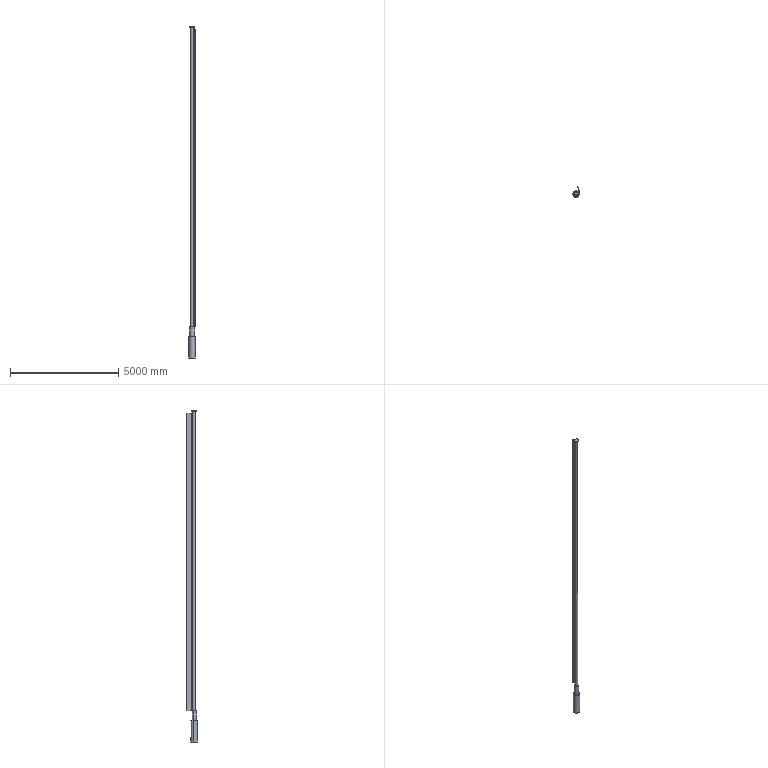Part | SolidWorks | features ICE 9, Extrusion 1 | 1 solid | 27 faces | box 300 x 474.612 x 15314 mm | volume 388904585 mm3 | plane 19 | cylinder 8 | commonest cylinder face diameters 200 x4 300 x2 100 x1 117.35 x1
STEP:
#1=CARTESIAN_POINT('',(-100.,0.,-14264.));
#2=VERTEX_POINT('',#1);
#3=CARTESIAN_POINT('',(100.,0.,-14264.));
#4=VERTEX_POINT('',#3);
#5=CARTESIAN_POINT('',(0.,0.,-14264.));
#6=DIRECTION('',(0.,0.,-1.));
#7=DIRECTION('',(-1.,0.,0.));
#8=AXIS2_PLACEMENT_3D('',#5,#6,#7);
#9=CIRCLE('',#8,100.);
#10=EDGE_CURVE('',#2,#4,#9,.T.);
#11=ORIENTED_EDGE('',*,*,#10,.F.);
#12=CARTESIAN_POINT('',(-100.,0.,-13824.));
#13=VERTEX_POINT('',#12);
#14=CARTESIAN_POINT('',(-100.,0.,-14264.));
#15=DIRECTION('',(0.,0.,1.));
#16=VECTOR('',#15,1000.);
#17=LINE('',#14,#16);
#18=EDGE_CURVE('',#2,#13,#17,.T.);
#19=ORIENTED_EDGE('',*,*,#18,.T.);
#20=CARTESIAN_POINT('',(61.826,78.598,-13824.));
#21=VERTEX_POINT('',#20);
#22=CARTESIAN_POINT('',(0.,0.,-13824.));
#23=DIRECTION('',(0.,0.,-1.));
#24=DIRECTION('',(-1.,0.,0.));
#25=AXIS2_PLACEMENT_3D('',#22,#23,#24);
#26=CIRCLE('',#25,100.);
#27=EDGE_CURVE('',#13,#21,#26,.T.);
#28=ORIENTED_EDGE('',*,*,#27,.T.);
#29=CARTESIAN_POINT('',(96.233,27.187,-13824.));
#30=VERTEX_POINT('',#29);
#31=CARTESIAN_POINT('',(0.,0.,-13824.));
#32=DIRECTION('',(0.,0.,-1.));
#33=DIRECTION('',(-1.,0.,0.));
#34=AXIS2_PLACEMENT_3D('',#31,#32,#33);
#35=CIRCLE('',#34,100.);
#36=EDGE_CURVE('',#21,#30,#35,.T.);
#37=ORIENTED_EDGE('',*,*,#36,.T.);
#38=CARTESIAN_POINT('',(100.,0.,-13824.));
#39=VERTEX_POINT('',#38);
#40=CARTESIAN_POINT('',(0.,0.,-13824.));
#41=DIRECTION('',(0.,0.,-1.));
#42=DIRECTION('',(-1.,0.,0.));
#43=AXIS2_PLACEMENT_3D('',#40,#41,#42);
#44=CIRCLE('',#43,100.);
#45=EDGE_CURVE('',#30,#39,#44,.T.);
#46=ORIENTED_EDGE('',*,*,#45,.T.);
#47=CARTESIAN_POINT('',(100.,0.,-14264.));
#48=DIRECTION('',(0.,0.,1.));
#49=VECTOR('',#48,1000.);
#50=LINE('',#47,#49);
#51=EDGE_CURVE('',#4,#39,#50,.T.);
#52=ORIENTED_EDGE('',*,*,#51,.F.);
#53=EDGE_LOOP('',(#11,#19,#28,#37,#46,#52));
#54=FACE_OUTER_BOUND('',#53,.T.);
#55=CARTESIAN_POINT('',(0.,0.,-14264.));
#56=DIRECTION('',(0.,0.,1.));
#57=DIRECTION('',(1.,0.,0.));
#58=AXIS2_PLACEMENT_3D('',#55,#56,#57);
#59=CYLINDRICAL_SURFACE('',#58,100.);
#60=ADVANCED_FACE('',(#54),#59,.T.);
#61=CARTESIAN_POINT('',(-100.,0.,50.));
#62=VERTEX_POINT('',#61);
#63=CARTESIAN_POINT('',(100.,0.,50.));
#64=VERTEX_POINT('',#63);
#65=CARTESIAN_POINT('',(0.,0.,50.));
#66=DIRECTION('',(0.,0.,-1.));
#67=DIRECTION('',(-1.,0.,0.));
#68=AXIS2_PLACEMENT_3D('',#65,#66,#67);
#69=CIRCLE('',#68,100.);
#70=EDGE_CURVE('',#62,#64,#69,.T.);
#71=ORIENTED_EDGE('',*,*,#70,.T.);
#72=CARTESIAN_POINT('',(100.,0.,0.));
#73=VERTEX_POINT('',#72);
#74=CARTESIAN_POINT('',(100.,0.,50.));
#75=DIRECTION('',(0.,0.,-1.));
#76=VECTOR('',#75,1000.);
#77=LINE('',#74,#76);
#78=EDGE_CURVE('',#64,#73,#77,.T.);
#79=ORIENTED_EDGE('',*,*,#78,.T.);
#80=CARTESIAN_POINT('',(96.233,27.187,0.));
#81=VERTEX_POINT('',#80);
#82=CARTESIAN_POINT('',(0.,0.,0.));
#83=DIRECTION('',(0.,0.,1.));
#84=DIRECTION('',(1.,0.,0.));
#85=AXIS2_PLACEMENT_3D('',#82,#83,#84);
#86=CIRCLE('',#85,100.);
#87=EDGE_CURVE('',#73,#81,#86,.T.);
#88=ORIENTED_EDGE('',*,*,#87,.T.);
#89=CARTESIAN_POINT('',(96.233,27.187,-100.));
#90=VERTEX_POINT('',#89);
#91=CARTESIAN_POINT('',(96.233,27.187,-100.));
#92=DIRECTION('',(0.,0.,1.));
#93=VECTOR('',#92,1000.);
#94=LINE('',#91,#93);
#95=EDGE_CURVE('',#90,#81,#94,.T.);
#96=ORIENTED_EDGE('',*,*,#95,.F.);
#97=CARTESIAN_POINT('',(61.826,78.598,-100.));
#98=VERTEX_POINT('',#97);
#99=CARTESIAN_POINT('',(0.,0.,-100.));
#100=DIRECTION('',(0.,0.,-1.));
#101=DIRECTION('',(1.,0.,0.));
#102=AXIS2_PLACEMENT_3D('',#99,#100,#101);
#103=CIRCLE('',#102,100.);
#104=EDGE_CURVE('',#98,#90,#103,.T.);
#105=ORIENTED_EDGE('',*,*,#104,.F.);
#106=CARTESIAN_POINT('',(61.826,78.598,0.));
#107=VERTEX_POINT('',#106);
#108=CARTESIAN_POINT('',(61.826,78.598,-100.));
#109=DIRECTION('',(0.,0.,1.));
#110=VECTOR('',#109,1000.);
#111=LINE('',#108,#110);
#112=EDGE_CURVE('',#98,#107,#111,.T.);
#113=ORIENTED_EDGE('',*,*,#112,.T.);
#114=CARTESIAN_POINT('',(-100.,0.,0.));
#115=VERTEX_POINT('',#114);
#116=CARTESIAN_POINT('',(0.,0.,0.));
#117=DIRECTION('',(0.,0.,1.));
#118=DIRECTION('',(1.,0.,0.));
#119=AXIS2_PLACEMENT_3D('',#116,#117,#118);
#120=CIRCLE('',#119,100.);
#121=EDGE_CURVE('',#107,#115,#120,.T.);
#122=ORIENTED_EDGE('',*,*,#121,.T.);
#123=CARTESIAN_POINT('',(-100.,0.,50.));
#124=DIRECTION('',(0.,0.,-1.));
#125=VECTOR('',#124,1000.);
#126=LINE('',#123,#125);
#127=EDGE_CURVE('',#62,#115,#126,.T.);
#128=ORIENTED_EDGE('',*,*,#127,.F.);
#129=EDGE_LOOP('',(#71,#79,#88,#96,#105,#113,#122,#128));
#130=FACE_OUTER_BOUND('',#129,.T.);
#131=CARTESIAN_POINT('',(0.,0.,50.));
#132=DIRECTION('',(0.,0.,-1.));
#133=DIRECTION('',(-1.,0.,0.));
#134=AXIS2_PLACEMENT_3D('',#131,#132,#133);
#135=CYLINDRICAL_SURFACE('',#134,100.);
#136=ADVANCED_FACE('',(#130),#135,.T.);
#137=CARTESIAN_POINT('',(-150.,0.,-15264.));
#138=VERTEX_POINT('',#137);
#139=CARTESIAN_POINT('',(-50.,141.421,-15264.));
#140=VERTEX_POINT('',#139);
#141=CARTESIAN_POINT('',(0.,0.,-15264.));
#142=DIRECTION('',(0.,0.,-1.));
#143=DIRECTION('',(-1.,0.,0.));
#144=AXIS2_PLACEMENT_3D('',#141,#142,#143);
#145=CIRCLE('',#144,150.);
#146=EDGE_CURVE('',#138,#140,#145,.T.);
#147=ORIENTED_EDGE('',*,*,#146,.F.);
#148=CARTESIAN_POINT('',(-150.,0.,-14264.));
#149=VERTEX_POINT('',#148);
#150=CARTESIAN_POINT('',(-150.,0.,-15264.));
#151=DIRECTION('',(0.,0.,1.));
#152=VECTOR('',#151,1000.);
#153=LINE('',#150,#152);
#154=EDGE_CURVE('',#138,#149,#153,.T.);
#155=ORIENTED_EDGE('',*,*,#154,.T.);
#156=CARTESIAN_POINT('',(150.,0.,-14264.));
#157=VERTEX_POINT('',#156);
#158=CARTESIAN_POINT('',(0.,0.,-14264.));
#159=DIRECTION('',(0.,0.,-1.));
#160=DIRECTION('',(-1.,0.,0.));
#161=AXIS2_PLACEMENT_3D('',#158,#159,#160);
#162=CIRCLE('',#161,150.);
#163=EDGE_CURVE('',#149,#157,#162,.T.);
#164=ORIENTED_EDGE('',*,*,#163,.T.);
#165=CARTESIAN_POINT('',(150.,0.,-15264.));
#166=VERTEX_POINT('',#165);
#167=CARTESIAN_POINT('',(150.,0.,-15264.));
#168=DIRECTION('',(0.,0.,1.));
#169=VECTOR('',#168,1000.);
#170=LINE('',#167,#169);
#171=EDGE_CURVE('',#166,#157,#170,.T.);
#172=ORIENTED_EDGE('',*,*,#171,.F.);
#173=CARTESIAN_POINT('',(50.,141.421,-15264.));
#174=VERTEX_POINT('',#173);
#175=CARTESIAN_POINT('',(0.,0.,-15264.));
#176=DIRECTION('',(0.,0.,-1.));
#177=DIRECTION('',(-1.,0.,0.));
#178=AXIS2_PLACEMENT_3D('',#175,#176,#177);
#179=CIRCLE('',#178,150.);
#180=EDGE_CURVE('',#174,#166,#179,.T.);
#181=ORIENTED_EDGE('',*,*,#180,.F.);
#182=CARTESIAN_POINT('',(50.,141.421,-15084.));
#183=VERTEX_POINT('',#182);
#184=CARTESIAN_POINT('',(50.,141.421,-15264.));
#185=DIRECTION('',(0.,0.,-1.));
#186=VECTOR('',#185,1000.);
#187=LINE('',#184,#186);
#188=EDGE_CURVE('',#183,#174,#187,.T.);
#189=ORIENTED_EDGE('',*,*,#188,.F.);
#190=CARTESIAN_POINT('',(-50.,141.421,-15084.));
#191=VERTEX_POINT('',#190);
#192=CARTESIAN_POINT('',(-50.,141.421,-15084.));
#193=CARTESIAN_POINT('',(-50.,141.421,-15080.672));
#194=CARTESIAN_POINT('',(-49.671,141.539,-15077.404));
#195=CARTESIAN_POINT('',(-48.708,141.872,-15072.589));
#196=CARTESIAN_POINT('',(-48.308,142.009,-15070.998));
#197=CARTESIAN_POINT('',(-47.588,142.251,-15068.634));
#198=CARTESIAN_POINT('',(-47.326,142.339,-15067.848));
#199=CARTESIAN_POINT('',(-46.768,142.523,-15066.297));
#200=CARTESIAN_POINT('',(-46.472,142.62,-15065.532));
#201=CARTESIAN_POINT('',(-44.899,143.129,-15061.757));
#202=CARTESIAN_POINT('',(-43.363,143.608,-15058.895));
#203=CARTESIAN_POINT('',(-41.098,144.261,-15055.511));
#204=CARTESIAN_POINT('',(-40.627,144.394,-15054.844));
#205=CARTESIAN_POINT('',(-39.651,144.665,-15053.529));
#206=CARTESIAN_POINT('',(-39.146,144.803,-15052.883));
#207=CARTESIAN_POINT('',(-37.593,145.217,-15050.994));
#208=CARTESIAN_POINT('',(-36.503,145.495,-15049.793));
#209=CARTESIAN_POINT('',(-33.072,146.328,-15046.361));
#210=CARTESIAN_POINT('',(-30.571,146.878,-15044.299));
#211=CARTESIAN_POINT('',(-26.479,147.651,-15041.555));
#212=CARTESIAN_POINT('',(-25.079,147.896,-15040.714));
#213=CARTESIAN_POINT('',(-22.212,148.353,-15039.175));
#214=CARTESIAN_POINT('',(-20.744,148.566,-15038.477));
#215=CARTESIAN_POINT('',(-17.741,148.955,-15037.225));
#216=CARTESIAN_POINT('',(-16.206,149.13,-15036.671));
#217=CARTESIAN_POINT('',(-13.849,149.361,-15035.949));
#218=CARTESIAN_POINT('',(-13.055,149.433,-15035.727));
#219=CARTESIAN_POINT('',(-11.448,149.565,-15035.321));
#220=CARTESIAN_POINT('',(-10.64,149.624,-15035.138));
#221=CARTESIAN_POINT('',(-6.6,149.89,-15034.328));
#222=CARTESIAN_POINT('',(-3.34,149.999,-15034.004));
#223=CARTESIAN_POINT('',(0.7688,150.,-15033.999));
#224=CARTESIAN_POINT('',(1.592,149.994,-15034.019));
#225=CARTESIAN_POINT('',(3.243,149.967,-15034.098));
#226=CARTESIAN_POINT('',(4.072,149.947,-15034.159));
#227=CARTESIAN_POINT('',(6.551,149.866,-15034.403));
#228=CARTESIAN_POINT('',(8.181,149.785,-15034.647));
#229=CARTESIAN_POINT('',(13.006,149.47,-15035.61));
#230=CARTESIAN_POINT('',(16.136,149.161,-15036.561));
#231=CARTESIAN_POINT('',(19.939,148.671,-15038.14));
#232=CARTESIAN_POINT('',(20.695,148.567,-15038.476));
#233=CARTESIAN_POINT('',(22.178,148.353,-15039.18));
#234=CARTESIAN_POINT('',(22.908,148.242,-15039.549));
#235=CARTESIAN_POINT('',(25.063,147.898,-15040.705));
#236=CARTESIAN_POINT('',(26.456,147.655,-15041.541));
#237=CARTESIAN_POINT('',(29.152,147.146,-15043.346));
#238=CARTESIAN_POINT('',(30.456,146.881,-15044.313));
#239=CARTESIAN_POINT('',(32.347,146.472,-15045.864));
#240=CARTESIAN_POINT('',(32.966,146.334,-15046.398));
#241=CARTESIAN_POINT('',(34.18,146.055,-15047.498));
#242=CARTESIAN_POINT('',(34.771,145.915,-15048.061));
#243=CARTESIAN_POINT('',(37.648,145.218,-15050.936));
#244=CARTESIAN_POINT('',(39.702,144.663,-15053.434));
#245=CARTESIAN_POINT('',(41.965,144.011,-15056.805));
#246=CARTESIAN_POINT('',(42.403,143.883,-15057.492));
#247=CARTESIAN_POINT('',(43.246,143.631,-15058.892));
#248=CARTESIAN_POINT('',(43.653,143.508,-15059.606));
#249=CARTESIAN_POINT('',(44.82,143.15,-15061.777));
#250=CARTESIAN_POINT('',(45.522,142.927,-15063.253));
#251=CARTESIAN_POINT('',(47.402,142.319,-15067.763));
#252=CARTESIAN_POINT('',(48.361,141.992,-15070.88));
#253=CARTESIAN_POINT('',(49.176,141.71,-15074.922));
#254=CARTESIAN_POINT('',(49.32,141.66,-15075.739));
#255=CARTESIAN_POINT('',(49.567,141.574,-15077.381));
#256=CARTESIAN_POINT('',(49.67,141.538,-15078.204));
#257=CARTESIAN_POINT('',(49.917,141.451,-15080.679));
#258=CARTESIAN_POINT('',(50.,141.421,-15082.336));
#259=CARTESIAN_POINT('',(50.,141.421,-15084.));
#260=B_SPLINE_CURVE_WITH_KNOTS('',3,(#192,#193,#194,#195,#196,#197,#198,#199,#200,#201,#202,#203,#204,#205,#206,#207,#208,#209,#210,#211,#212,#213,#214,#215,#216,#217,#218,#219,#220,#221,#222,#223,#224,#225,#226,#227,#228,#229,#230,#231,#232,#233,#234,#235,#236,#237,#238,#239,#240,#241,#242,#243,#244,#245,#246,#247,#248,#249,#250,#251,#252,#253,#254,#255,#256,#257,#258,#259),.UNSPECIFIED.,.F.,.F.,(4,2,2,2,2,2,2,2,2,2,2,2,2,2,2,2,2,2,2,2,2,2,2,2,2,2,2,2,2,2,2,2,2,4),(0.,0.009837,0.01476,0.01721,0.01967,0.02951,0.03197,0.03443,0.03935,0.04919,0.0541,0.05902,0.06394,0.0664,0.06886,0.0787,0.08116,0.08362,0.08853,0.09837,0.1008,0.1033,0.1082,0.1131,0.1156,0.118,0.1279,0.1303,0.1328,0.1377,0.1476,0.15,0.1525,0.1574),.UNSPECIFIED.);
#261=EDGE_CURVE('',#191,#183,#260,.T.);
#262=ORIENTED_EDGE('',*,*,#261,.F.);
#263=CARTESIAN_POINT('',(-50.,141.421,-15264.));
#264=DIRECTION('',(0.,0.,1.));
#265=VECTOR('',#264,1000.);
#266=LINE('',#263,#265);
#267=EDGE_CURVE('',#140,#191,#266,.T.);
#268=ORIENTED_EDGE('',*,*,#267,.F.);
#269=EDGE_LOOP('',(#147,#155,#164,#172,#181,#189,#262,#268));
#270=FACE_OUTER_BOUND('',#269,.T.);
#271=CARTESIAN_POINT('',(0.,0.,-15264.));
#272=DIRECTION('',(0.,0.,1.));
#273=DIRECTION('',(1.,0.,0.));
#274=AXIS2_PLACEMENT_3D('',#271,#272,#273);
#275=CYLINDRICAL_SURFACE('',#274,150.);
#276=ADVANCED_FACE('',(#270),#275,.T.);
#277=ORIENTED_EDGE('',*,*,#154,.F.);
#278=CARTESIAN_POINT('',(0.,0.,-15264.));
#279=DIRECTION('',(0.,0.,-1.));
#280=DIRECTION('',(-1.,0.,0.));
#281=AXIS2_PLACEMENT_3D('',#278,#279,#280);
#282=CIRCLE('',#281,150.);
#283=EDGE_CURVE('',#166,#138,#282,.T.);
#284=ORIENTED_EDGE('',*,*,#283,.F.);
#285=ORIENTED_EDGE('',*,*,#171,.T.);
#286=CARTESIAN_POINT('',(0.,0.,-14264.));
#287=DIRECTION('',(0.,0.,-1.));
#288=DIRECTION('',(-1.,0.,0.));
#289=AXIS2_PLACEMENT_3D('',#286,#287,#288);
#290=CIRCLE('',#289,150.);
#291=EDGE_CURVE('',#157,#149,#290,.T.);
#292=ORIENTED_EDGE('',*,*,#291,.T.);
#293=EDGE_LOOP('',(#277,#284,#285,#292));
#294=FACE_OUTER_BOUND('',#293,.T.);
#295=CARTESIAN_POINT('',(0.,0.,-15264.));
#296=DIRECTION('',(0.,0.,1.));
#297=DIRECTION('',(1.,0.,0.));
#298=AXIS2_PLACEMENT_3D('',#295,#296,#297);
#299=CYLINDRICAL_SURFACE('',#298,150.);
#300=ADVANCED_FACE('',(#294),#299,.T.);
#301=ORIENTED_EDGE('',*,*,#180,.T.);
#302=ORIENTED_EDGE('',*,*,#283,.T.);
#303=ORIENTED_EDGE('',*,*,#146,.T.);
#304=CARTESIAN_POINT('',(-50.,65.,-15264.));
#305=VERTEX_POINT('',#304);
#306=CARTESIAN_POINT('',(-50.,0.,-15264.));
#307=DIRECTION('',(0.,-1.,0.));
#308=VECTOR('',#307,1000.);
#309=LINE('',#306,#308);
#310=EDGE_CURVE('',#140,#305,#309,.T.);
#311=ORIENTED_EDGE('',*,*,#310,.T.);
#312=CARTESIAN_POINT('',(50.,65.,-15264.));
#313=VERTEX_POINT('',#312);
#314=CARTESIAN_POINT('',(0.,65.,-15264.));
#315=DIRECTION('',(1.,0.,0.));
#316=VECTOR('',#315,1000.);
#317=LINE('',#314,#316);
#318=EDGE_CURVE('',#305,#313,#317,.T.);
#319=ORIENTED_EDGE('',*,*,#318,.T.);
#320=CARTESIAN_POINT('',(50.,0.,-15264.));
#321=DIRECTION('',(0.,1.,0.));
#322=VECTOR('',#321,1000.);
#323=LINE('',#320,#322);
#324=EDGE_CURVE('',#313,#174,#323,.T.);
#325=ORIENTED_EDGE('',*,*,#324,.T.);
#326=EDGE_LOOP('',(#301,#302,#303,#311,#319,#325));
#327=FACE_OUTER_BOUND('',#326,.T.);
#328=CARTESIAN_POINT('',(0.,0.,-15264.));
#329=DIRECTION('',(0.,0.,-1.));
#330=DIRECTION('',(-1.,0.,0.));
#331=AXIS2_PLACEMENT_3D('',#328,#329,#330);
#332=PLANE('',#331);
#333=ADVANCED_FACE('',(#327),#332,.T.);
#334=CARTESIAN_POINT('',(127.239,110.96,-100.));
#335=VERTEX_POINT('',#334);
#336=CARTESIAN_POINT('',(127.239,110.96,-100.));
#337=DIRECTION('',(-0.8963,-0.4434,0.));
#338=VECTOR('',#337,1000.);
#339=LINE('',#336,#338);
#340=EDGE_CURVE('',#335,#98,#339,.T.);
#341=ORIENTED_EDGE('',*,*,#340,.F.);
#342=CARTESIAN_POINT('',(127.239,110.96,-13824.));
#343=VERTEX_POINT('',#342);
#344=CARTESIAN_POINT('',(127.239,110.96,-13824.));
#345=DIRECTION('',(0.,0.,1.));
#346=VECTOR('',#345,1000.);
#347=LINE('',#344,#346);
#348=EDGE_CURVE('',#343,#335,#347,.T.);
#349=ORIENTED_EDGE('',*,*,#348,.F.);
#350=CARTESIAN_POINT('',(127.239,110.96,-13824.));
#351=DIRECTION('',(0.8963,0.4434,0.));
#352=VECTOR('',#351,1000.);
#353=LINE('',#350,#352);
#354=EDGE_CURVE('',#21,#343,#353,.T.);
#355=ORIENTED_EDGE('',*,*,#354,.F.);
#356=CARTESIAN_POINT('',(61.826,78.598,-13824.));
#357=DIRECTION('',(0.,0.,1.));
#358=VECTOR('',#357,1000.);
#359=LINE('',#356,#358);
#360=EDGE_CURVE('',#21,#98,#359,.T.);
#361=ORIENTED_EDGE('',*,*,#360,.T.);
#362=EDGE_LOOP('',(#341,#349,#355,#361));
#363=FACE_OUTER_BOUND('',#362,.T.);
#364=CARTESIAN_POINT('',(127.239,110.96,-13824.));
#365=DIRECTION('',(0.4434,-0.8963,0.));
#366=DIRECTION('',(0.8963,0.4434,0.));
#367=AXIS2_PLACEMENT_3D('',#364,#365,#366);
#368=PLANE('',#367);
#369=ADVANCED_FACE('',(#363),#368,.F.);
#370=CARTESIAN_POINT('',(106.547,286.808,-100.));
#371=VERTEX_POINT('',#370);
#372=CARTESIAN_POINT('',(106.547,286.808,-100.));
#373=DIRECTION('',(0.1169,-0.9931,0.));
#374=VECTOR('',#373,1000.);
#375=LINE('',#372,#374);
#376=EDGE_CURVE('',#371,#335,#375,.T.);
#377=ORIENTED_EDGE('',*,*,#376,.F.);
#378=CARTESIAN_POINT('',(106.547,286.808,-13824.));
#379=VERTEX_POINT('',#378);
#380=CARTESIAN_POINT('',(106.547,286.808,-13824.));
#381=DIRECTION('',(0.,0.,1.));
#382=VECTOR('',#381,1000.);
#383=LINE('',#380,#382);
#384=EDGE_CURVE('',#379,#371,#383,.T.);
#385=ORIENTED_EDGE('',*,*,#384,.F.);
#386=CARTESIAN_POINT('',(106.547,286.808,-13824.));
#387=DIRECTION('',(-0.1169,0.9931,0.));
#388=VECTOR('',#387,1000.);
#389=LINE('',#386,#388);
#390=EDGE_CURVE('',#343,#379,#389,.T.);
#391=ORIENTED_EDGE('',*,*,#390,.F.);
#392=ORIENTED_EDGE('',*,*,#348,.T.);
#393=EDGE_LOOP('',(#377,#385,#391,#392));
#394=FACE_OUTER_BOUND('',#393,.T.);
#395=CARTESIAN_POINT('',(106.547,286.808,-13824.));
#396=DIRECTION('',(0.9931,0.1169,0.));
#397=DIRECTION('',(-0.1169,0.9931,0.));
#398=AXIS2_PLACEMENT_3D('',#395,#396,#397);
#399=PLANE('',#398);
#400=ADVANCED_FACE('',(#394),#399,.F.);
#401=CARTESIAN_POINT('',(53.816,324.612,-100.));
#402=VERTEX_POINT('',#401);
#403=CARTESIAN_POINT('',(53.816,324.612,-100.));
#404=DIRECTION('',(0.8127,-0.5827,0.));
#405=VECTOR('',#404,1000.);
#406=LINE('',#403,#405);
#407=EDGE_CURVE('',#402,#371,#406,.T.);
#408=ORIENTED_EDGE('',*,*,#407,.F.);
#409=CARTESIAN_POINT('',(53.816,324.612,-13824.));
#410=VERTEX_POINT('',#409);
#411=CARTESIAN_POINT('',(53.816,324.612,-13824.));
#412=DIRECTION('',(0.,0.,1.));
#413=VECTOR('',#412,1000.);
#414=LINE('',#411,#413);
#415=EDGE_CURVE('',#410,#402,#414,.T.);
#416=ORIENTED_EDGE('',*,*,#415,.F.);
#417=CARTESIAN_POINT('',(69.836,313.127,-13824.));
#418=DIRECTION('',(-0.8127,0.5827,0.));
#419=VECTOR('',#418,1000.);
#420=LINE('',#417,#419);
#421=EDGE_CURVE('',#379,#410,#420,.T.);
#422=ORIENTED_EDGE('',*,*,#421,.F.);
#423=ORIENTED_EDGE('',*,*,#384,.T.);
#424=EDGE_LOOP('',(#408,#416,#422,#423));
#425=FACE_OUTER_BOUND('',#424,.T.);
#426=CARTESIAN_POINT('',(53.816,324.612,-13824.));
#427=DIRECTION('',(0.5827,0.8127,0.));
#428=DIRECTION('',(-0.8127,0.5827,0.));
#429=AXIS2_PLACEMENT_3D('',#426,#427,#428);
#430=PLANE('',#429);
#431=ADVANCED_FACE('',(#425),#430,.F.);
#432=CARTESIAN_POINT('',(85.855,324.612,-100.));
#433=VERTEX_POINT('',#432);
#434=CARTESIAN_POINT('',(85.855,324.612,-100.));
#435=DIRECTION('',(-1.,0.,0.));
#436=VECTOR('',#435,1000.);
#437=LINE('',#434,#436);
#438=EDGE_CURVE('',#433,#402,#437,.T.);
#439=ORIENTED_EDGE('',*,*,#438,.F.);
#440=CARTESIAN_POINT('',(85.855,324.612,-13824.));
#441=VERTEX_POINT('',#440);
#442=CARTESIAN_POINT('',(85.855,324.612,-13824.));
#443=DIRECTION('',(0.,0.,1.));
#444=VECTOR('',#443,1000.);
#445=LINE('',#442,#444);
#446=EDGE_CURVE('',#441,#433,#445,.T.);
#447=ORIENTED_EDGE('',*,*,#446,.F.);
#448=CARTESIAN_POINT('',(85.855,324.612,-13824.));
#449=DIRECTION('',(1.,0.,0.));
#450=VECTOR('',#449,1000.);
#451=LINE('',#448,#450);
#452=EDGE_CURVE('',#410,#441,#451,.T.);
#453=ORIENTED_EDGE('',*,*,#452,.F.);
#454=ORIENTED_EDGE('',*,*,#415,.T.);
#455=EDGE_LOOP('',(#439,#447,#453,#454));
#456=FACE_OUTER_BOUND('',#455,.T.);
#457=CARTESIAN_POINT('',(85.855,324.612,-13824.));
#458=DIRECTION('',(0.,-1.,0.));
#459=DIRECTION('',(0.,0.,-1.));
#460=AXIS2_PLACEMENT_3D('',#457,#458,#459);
#461=PLANE('',#460);
#462=ADVANCED_FACE('',(#456),#461,.F.);
#463=CARTESIAN_POINT('',(127.239,294.943,-100.));
#464=VERTEX_POINT('',#463);
#465=CARTESIAN_POINT('',(127.239,294.943,-100.));
#466=DIRECTION('',(-0.8127,0.5827,0.));
#467=VECTOR('',#466,1000.);
#468=LINE('',#465,#467);
#469=EDGE_CURVE('',#464,#433,#468,.T.);
#470=ORIENTED_EDGE('',*,*,#469,.F.);
#471=CARTESIAN_POINT('',(127.239,294.943,-13824.));
#472=VERTEX_POINT('',#471);
#473=CARTESIAN_POINT('',(127.239,294.943,-13824.));
#474=DIRECTION('',(0.,0.,1.));
#475=VECTOR('',#474,1000.);
#476=LINE('',#473,#475);
#477=EDGE_CURVE('',#472,#464,#476,.T.);
#478=ORIENTED_EDGE('',*,*,#477,.F.);
#479=CARTESIAN_POINT('',(127.239,294.943,-13824.));
#480=DIRECTION('',(0.8127,-0.5827,0.));
#481=VECTOR('',#480,1000.);
#482=LINE('',#479,#481);
#483=EDGE_CURVE('',#441,#472,#482,.T.);
#484=ORIENTED_EDGE('',*,*,#483,.F.);
#485=ORIENTED_EDGE('',*,*,#446,.T.);
#486=EDGE_LOOP('',(#470,#478,#484,#485));
#487=FACE_OUTER_BOUND('',#486,.T.);
#488=CARTESIAN_POINT('',(127.239,294.943,-13824.));
#489=DIRECTION('',(-0.5827,-0.8127,0.));
#490=DIRECTION('',(0.8127,-0.5827,0.));
#491=AXIS2_PLACEMENT_3D('',#488,#489,#490);
#492=PLANE('',#491);
#493=ADVANCED_FACE('',(#487),#492,.F.);
#494=CARTESIAN_POINT('',(146.429,97.202,-100.));
#495=VERTEX_POINT('',#494);
#496=CARTESIAN_POINT('',(146.429,97.202,-100.));
#497=DIRECTION('',(-0.09659,0.9953,0.));
#498=VECTOR('',#497,1000.);
#499=LINE('',#496,#498);
#500=EDGE_CURVE('',#495,#464,#499,.T.);
#501=ORIENTED_EDGE('',*,*,#500,.F.);
#502=CARTESIAN_POINT('',(146.429,97.202,-13824.));
#503=VERTEX_POINT('',#502);
#504=CARTESIAN_POINT('',(146.429,97.202,-13824.));
#505=DIRECTION('',(0.,0.,1.));
#506=VECTOR('',#505,1000.);
#507=LINE('',#504,#506);
#508=EDGE_CURVE('',#503,#495,#507,.T.);
#509=ORIENTED_EDGE('',*,*,#508,.F.);
#510=CARTESIAN_POINT('',(146.429,97.202,-13824.));
#511=DIRECTION('',(0.09659,-0.9953,0.));
#512=VECTOR('',#511,1000.);
#513=LINE('',#510,#512);
#514=EDGE_CURVE('',#472,#503,#513,.T.);
#515=ORIENTED_EDGE('',*,*,#514,.F.);
#516=ORIENTED_EDGE('',*,*,#477,.T.);
#517=EDGE_LOOP('',(#501,#509,#515,#516));
#518=FACE_OUTER_BOUND('',#517,.T.);
#519=CARTESIAN_POINT('',(146.429,97.202,-13824.));
#520=DIRECTION('',(-0.9953,-0.09659,0.));
#521=DIRECTION('',(0.09659,-0.9953,0.));
#522=AXIS2_PLACEMENT_3D('',#519,#520,#521);
#523=PLANE('',#522);
#524=ADVANCED_FACE('',(#518),#523,.F.);
#525=CARTESIAN_POINT('',(96.233,27.187,-100.));
#526=DIRECTION('',(0.5827,0.8127,0.));
#527=VECTOR('',#526,1000.);
#528=LINE('',#525,#527);
#529=EDGE_CURVE('',#90,#495,#528,.T.);
#530=ORIENTED_EDGE('',*,*,#529,.F.);
#531=CARTESIAN_POINT('',(96.233,27.187,-13824.));
#532=DIRECTION('',(0.,0.,1.));
#533=VECTOR('',#532,1000.);
#534=LINE('',#531,#533);
#535=EDGE_CURVE('',#30,#90,#534,.T.);
#536=ORIENTED_EDGE('',*,*,#535,.F.);
#537=CARTESIAN_POINT('',(96.233,27.187,-13824.));
#538=DIRECTION('',(-0.5827,-0.8127,0.));
#539=VECTOR('',#538,1000.);
#540=LINE('',#537,#539);
#541=EDGE_CURVE('',#503,#30,#540,.T.);
#542=ORIENTED_EDGE('',*,*,#541,.F.);
#543=ORIENTED_EDGE('',*,*,#508,.T.);
#544=EDGE_LOOP('',(#530,#536,#542,#543));
#545=FACE_OUTER_BOUND('',#544,.T.);
#546=CARTESIAN_POINT('',(96.233,27.187,-13824.));
#547=DIRECTION('',(-0.8127,0.5827,0.));
#548=DIRECTION('',(-0.5827,-0.8127,0.));
#549=AXIS2_PLACEMENT_3D('',#546,#547,#548);
#550=PLANE('',#549);
#551=ADVANCED_FACE('',(#545),#550,.F.);
#552=ORIENTED_EDGE('',*,*,#78,.F.);
#553=CARTESIAN_POINT('',(0.,0.,50.));
#554=DIRECTION('',(0.,0.,-1.));
#555=DIRECTION('',(-1.,0.,0.));
#556=AXIS2_PLACEMENT_3D('',#553,#554,#555);
#557=CIRCLE('',#556,100.);
#558=EDGE_CURVE('',#64,#62,#557,.T.);
#559=ORIENTED_EDGE('',*,*,#558,.T.);
#560=ORIENTED_EDGE('',*,*,#127,.T.);
#561=CARTESIAN_POINT('',(0.,0.,0.));
#562=DIRECTION('',(0.,0.,1.));
#563=DIRECTION('',(1.,0.,0.));
#564=AXIS2_PLACEMENT_3D('',#561,#562,#563);
#565=CIRCLE('',#564,100.);
#566=EDGE_CURVE('',#115,#73,#565,.T.);
#567=ORIENTED_EDGE('',*,*,#566,.T.);
#568=EDGE_LOOP('',(#552,#559,#560,#567));
#569=FACE_OUTER_BOUND('',#568,.T.);
#570=CARTESIAN_POINT('',(0.,0.,50.));
#571=DIRECTION('',(0.,0.,-1.));
#572=DIRECTION('',(-1.,0.,0.));
#573=AXIS2_PLACEMENT_3D('',#570,#571,#572);
#574=CYLINDRICAL_SURFACE('',#573,100.);
#575=ADVANCED_FACE('',(#569),#574,.T.);
#576=CARTESIAN_POINT('',(48.187,-33.477,0.));
#577=VERTEX_POINT('',#576);
#578=CARTESIAN_POINT('',(96.233,27.187,0.));
#579=DIRECTION('',(-0.6209,-0.7839,0.));
#580=VECTOR('',#579,1000.);
#581=LINE('',#578,#580);
#582=EDGE_CURVE('',#81,#577,#581,.T.);
#583=ORIENTED_EDGE('',*,*,#582,.F.);
#584=ORIENTED_EDGE('',*,*,#87,.F.);
#585=ORIENTED_EDGE('',*,*,#566,.F.);
#586=ORIENTED_EDGE('',*,*,#121,.F.);
#587=CARTESIAN_POINT('',(0.,58.675,0.));
#588=VERTEX_POINT('',#587);
#589=CARTESIAN_POINT('',(61.826,78.598,0.));
#590=DIRECTION('',(0.9518,0.3067,0.));
#591=VECTOR('',#590,1000.);
#592=LINE('',#589,#591);
#593=EDGE_CURVE('',#588,#107,#592,.T.);
#594=ORIENTED_EDGE('',*,*,#593,.F.);
#595=CARTESIAN_POINT('',(0.,0.,0.));
#596=DIRECTION('',(0.,0.,-1.));
#597=DIRECTION('',(-1.,0.,0.));
#598=AXIS2_PLACEMENT_3D('',#595,#596,#597);
#599=CIRCLE('',#598,58.675);
#600=EDGE_CURVE('',#577,#588,#599,.T.);
#601=ORIENTED_EDGE('',*,*,#600,.F.);
#602=EDGE_LOOP('',(#583,#584,#585,#586,#594,#601));
#603=FACE_OUTER_BOUND('',#602,.T.);
#604=CARTESIAN_POINT('',(0.,0.,0.));
#605=DIRECTION('',(0.,0.,1.));
#606=DIRECTION('',(1.,0.,0.));
#607=AXIS2_PLACEMENT_3D('',#604,#605,#606);
#608=PLANE('',#607);
#609=ADVANCED_FACE('',(#603),#608,.F.);
#610=ORIENTED_EDGE('',*,*,#582,.T.);
#611=CARTESIAN_POINT('',(48.187,-33.477,-13824.));
#612=VERTEX_POINT('',#611);
#613=CARTESIAN_POINT('',(48.187,-33.477,-13824.));
#614=DIRECTION('',(0.,0.,1.));
#615=VECTOR('',#614,1000.);
#616=LINE('',#613,#615);
#617=EDGE_CURVE('',#612,#577,#616,.T.);
#618=ORIENTED_EDGE('',*,*,#617,.F.);
#619=CARTESIAN_POINT('',(96.233,27.187,-13824.));
#620=DIRECTION('',(-0.6209,-0.7839,0.));
#621=VECTOR('',#620,1000.);
#622=LINE('',#619,#621);
#623=EDGE_CURVE('',#30,#612,#622,.T.);
#624=ORIENTED_EDGE('',*,*,#623,.F.);
#625=ORIENTED_EDGE('',*,*,#535,.T.);
#626=ORIENTED_EDGE('',*,*,#95,.T.);
#627=EDGE_LOOP('',(#610,#618,#624,#625,#626));
#628=FACE_OUTER_BOUND('',#627,.T.);
#629=CARTESIAN_POINT('',(96.233,27.187,-13824.));
#630=DIRECTION('',(-0.7839,0.6209,0.));
#631=DIRECTION('',(-0.6209,-0.7839,0.));
#632=AXIS2_PLACEMENT_3D('',#629,#630,#631);
#633=PLANE('',#632);
#634=ADVANCED_FACE('',(#628),#633,.F.);
#635=ORIENTED_EDGE('',*,*,#600,.T.);
#636=CARTESIAN_POINT('',(0.,58.675,-13824.));
#637=VERTEX_POINT('',#636);
#638=CARTESIAN_POINT('',(0.,58.675,-13824.));
#639=DIRECTION('',(0.,0.,1.));
#640=VECTOR('',#639,1000.);
#641=LINE('',#638,#640);
#642=EDGE_CURVE('',#637,#588,#641,.T.);
#643=ORIENTED_EDGE('',*,*,#642,.F.);
#644=CARTESIAN_POINT('',(0.,0.,-13824.));
#645=DIRECTION('',(0.,0.,-1.));
#646=DIRECTION('',(-1.,0.,0.));
#647=AXIS2_PLACEMENT_3D('',#644,#645,#646);
#648=CIRCLE('',#647,58.675);
#649=EDGE_CURVE('',#612,#637,#648,.T.);
#650=ORIENTED_EDGE('',*,*,#649,.F.);
#651=ORIENTED_EDGE('',*,*,#617,.T.);
#652=EDGE_LOOP('',(#635,#643,#650,#651));
#653=FACE_OUTER_BOUND('',#652,.T.);
#654=CARTESIAN_POINT('',(0.,0.,-13824.));
#655=DIRECTION('',(0.,0.,1.));
#656=DIRECTION('',(1.,0.,0.));
#657=AXIS2_PLACEMENT_3D('',#654,#655,#656);
#658=CYLINDRICAL_SURFACE('',#657,58.675);
#659=ADVANCED_FACE('',(#653),#658,.T.);
#660=ORIENTED_EDGE('',*,*,#593,.T.);
#661=ORIENTED_EDGE('',*,*,#112,.F.);
#662=ORIENTED_EDGE('',*,*,#360,.F.);
#663=CARTESIAN_POINT('',(61.826,78.598,-13824.));
#664=DIRECTION('',(0.9518,0.3067,0.));
#665=VECTOR('',#664,1000.);
#666=LINE('',#663,#665);
#667=EDGE_CURVE('',#637,#21,#666,.T.);
#668=ORIENTED_EDGE('',*,*,#667,.F.);
#669=ORIENTED_EDGE('',*,*,#642,.T.);
#670=EDGE_LOOP('',(#660,#661,#662,#668,#669));
#671=FACE_OUTER_BOUND('',#670,.T.);
#672=CARTESIAN_POINT('',(61.826,78.598,-13824.));
#673=DIRECTION('',(0.3067,-0.9518,0.));
#674=DIRECTION('',(0.9518,0.3067,0.));
#675=AXIS2_PLACEMENT_3D('',#672,#673,#674);
#676=PLANE('',#675);
#677=ADVANCED_FACE('',(#671),#676,.F.);
#678=ORIENTED_EDGE('',*,*,#36,.F.);
#679=ORIENTED_EDGE('',*,*,#354,.T.);
#680=ORIENTED_EDGE('',*,*,#390,.T.);
#681=ORIENTED_EDGE('',*,*,#421,.T.);
#682=ORIENTED_EDGE('',*,*,#452,.T.);
#683=ORIENTED_EDGE('',*,*,#483,.T.);
#684=ORIENTED_EDGE('',*,*,#514,.T.);
#685=ORIENTED_EDGE('',*,*,#541,.T.);
#686=EDGE_LOOP('',(#678,#679,#680,#681,#682,#683,#684,#685));
#687=FACE_OUTER_BOUND('',#686,.T.);
#688=CARTESIAN_POINT('',(0.,0.,-13824.));
#689=DIRECTION('',(0.,0.,-1.));
#690=DIRECTION('',(-1.,0.,0.));
#691=AXIS2_PLACEMENT_3D('',#688,#689,#690);
#692=PLANE('',#691);
#693=ADVANCED_FACE('',(#687),#692,.T.);
#694=ORIENTED_EDGE('',*,*,#45,.F.);
#695=ORIENTED_EDGE('',*,*,#623,.T.);
#696=ORIENTED_EDGE('',*,*,#649,.T.);
#697=ORIENTED_EDGE('',*,*,#667,.T.);
#698=ORIENTED_EDGE('',*,*,#27,.F.);
#699=CARTESIAN_POINT('',(0.,0.,-13824.));
#700=DIRECTION('',(0.,0.,-1.));
#701=DIRECTION('',(-1.,0.,0.));
#702=AXIS2_PLACEMENT_3D('',#699,#700,#701);
#703=CIRCLE('',#702,100.);
#704=EDGE_CURVE('',#39,#13,#703,.T.);
#705=ORIENTED_EDGE('',*,*,#704,.F.);
#706=EDGE_LOOP('',(#694,#695,#696,#697,#698,#705));
#707=FACE_OUTER_BOUND('',#706,.T.);
#708=CARTESIAN_POINT('',(0.,0.,-13824.));
#709=DIRECTION('',(0.,0.,-1.));
#710=DIRECTION('',(-1.,0.,0.));
#711=AXIS2_PLACEMENT_3D('',#708,#709,#710);
#712=PLANE('',#711);
#713=ADVANCED_FACE('',(#707),#712,.F.);
#714=ORIENTED_EDGE('',*,*,#18,.F.);
#715=CARTESIAN_POINT('',(0.,0.,-14264.));
#716=DIRECTION('',(0.,0.,-1.));
#717=DIRECTION('',(-1.,0.,0.));
#718=AXIS2_PLACEMENT_3D('',#715,#716,#717);
#719=CIRCLE('',#718,100.);
#720=EDGE_CURVE('',#4,#2,#719,.T.);
#721=ORIENTED_EDGE('',*,*,#720,.F.);
#722=ORIENTED_EDGE('',*,*,#51,.T.);
#723=ORIENTED_EDGE('',*,*,#704,.T.);
#724=EDGE_LOOP('',(#714,#721,#722,#723));
#725=FACE_OUTER_BOUND('',#724,.T.);
#726=CARTESIAN_POINT('',(0.,0.,-14264.));
#727=DIRECTION('',(0.,0.,1.));
#728=DIRECTION('',(1.,0.,0.));
#729=AXIS2_PLACEMENT_3D('',#726,#727,#728);
#730=CYLINDRICAL_SURFACE('',#729,100.);
#731=ADVANCED_FACE('',(#725),#730,.T.);
#732=ORIENTED_EDGE('',*,*,#104,.T.);
#733=ORIENTED_EDGE('',*,*,#529,.T.);
#734=ORIENTED_EDGE('',*,*,#500,.T.);
#735=ORIENTED_EDGE('',*,*,#469,.T.);
#736=ORIENTED_EDGE('',*,*,#438,.T.);
#737=ORIENTED_EDGE('',*,*,#407,.T.);
#738=ORIENTED_EDGE('',*,*,#376,.T.);
#739=ORIENTED_EDGE('',*,*,#340,.T.);
#740=EDGE_LOOP('',(#732,#733,#734,#735,#736,#737,#738,#739));
#741=FACE_OUTER_BOUND('',#740,.T.);
#742=CARTESIAN_POINT('',(0.,0.,-100.));
#743=DIRECTION('',(0.,0.,1.));
#744=DIRECTION('',(1.,0.,0.));
#745=AXIS2_PLACEMENT_3D('',#742,#743,#744);
#746=PLANE('',#745);
#747=ADVANCED_FACE('',(#741),#746,.T.);
#748=ORIENTED_EDGE('',*,*,#720,.T.);
#749=ORIENTED_EDGE('',*,*,#10,.T.);
#750=EDGE_LOOP('',(#748,#749));
#751=FACE_BOUND('',#750,.T.);
#752=ORIENTED_EDGE('',*,*,#291,.F.);
#753=ORIENTED_EDGE('',*,*,#163,.F.);
#754=EDGE_LOOP('',(#752,#753));
#755=FACE_OUTER_BOUND('',#754,.T.);
#756=CARTESIAN_POINT('',(0.,0.,-14264.));
#757=DIRECTION('',(0.,0.,-1.));
#758=DIRECTION('',(-1.,0.,0.));
#759=AXIS2_PLACEMENT_3D('',#756,#757,#758);
#760=PLANE('',#759);
#761=ADVANCED_FACE('',(#751,#755),#760,.F.);
#762=ORIENTED_EDGE('',*,*,#261,.T.);
#763=CARTESIAN_POINT('',(50.,65.,-15084.));
#764=VERTEX_POINT('',#763);
#765=CARTESIAN_POINT('',(50.,365.,-15084.));
#766=DIRECTION('',(0.,-1.,0.));
#767=VECTOR('',#766,1000.);
#768=LINE('',#765,#767);
#769=EDGE_CURVE('',#183,#764,#768,.T.);
#770=ORIENTED_EDGE('',*,*,#769,.T.);
#771=CARTESIAN_POINT('',(-50.,65.,-15084.));
#772=VERTEX_POINT('',#771);
#773=CARTESIAN_POINT('',(0.,65.,-15084.));
#774=DIRECTION('',(0.,1.,0.));
#775=DIRECTION('',(0.,0.,1.));
#776=AXIS2_PLACEMENT_3D('',#773,#774,#775);
#777=CIRCLE('',#776,50.);
#778=EDGE_CURVE('',#772,#764,#777,.T.);
#779=ORIENTED_EDGE('',*,*,#778,.F.);
#780=CARTESIAN_POINT('',(-50.,365.,-15084.));
#781=DIRECTION('',(0.,-1.,0.));
#782=VECTOR('',#781,1000.);
#783=LINE('',#780,#782);
#784=EDGE_CURVE('',#191,#772,#783,.T.);
#785=ORIENTED_EDGE('',*,*,#784,.F.);
#786=EDGE_LOOP('',(#762,#770,#779,#785));
#787=FACE_OUTER_BOUND('',#786,.T.);
#788=CARTESIAN_POINT('',(0.,365.,-15084.));
#789=DIRECTION('',(0.,-1.,0.));
#790=DIRECTION('',(0.,0.,-1.));
#791=AXIS2_PLACEMENT_3D('',#788,#789,#790);
#792=CYLINDRICAL_SURFACE('',#791,50.);
#793=ADVANCED_FACE('',(#787),#792,.F.);
#794=ORIENTED_EDGE('',*,*,#267,.T.);
#795=ORIENTED_EDGE('',*,*,#784,.T.);
#796=CARTESIAN_POINT('',(-50.,65.,-15384.));
#797=DIRECTION('',(0.,0.,1.));
#798=VECTOR('',#797,1000.);
#799=LINE('',#796,#798);
#800=EDGE_CURVE('',#305,#772,#799,.T.);
#801=ORIENTED_EDGE('',*,*,#800,.F.);
#802=ORIENTED_EDGE('',*,*,#310,.F.);
#803=EDGE_LOOP('',(#794,#795,#801,#802));
#804=FACE_OUTER_BOUND('',#803,.T.);
#805=CARTESIAN_POINT('',(-50.,365.,-15384.));
#806=DIRECTION('',(1.,0.,0.));
#807=DIRECTION('',(0.,0.,-1.));
#808=AXIS2_PLACEMENT_3D('',#805,#806,#807);
#809=PLANE('',#808);
#810=ADVANCED_FACE('',(#804),#809,.T.);
#811=ORIENTED_EDGE('',*,*,#188,.T.);
#812=ORIENTED_EDGE('',*,*,#324,.F.);
#813=CARTESIAN_POINT('',(50.,65.,-15384.));
#814=DIRECTION('',(0.,0.,-1.));
#815=VECTOR('',#814,1000.);
#816=LINE('',#813,#815);
#817=EDGE_CURVE('',#764,#313,#816,.T.);
#818=ORIENTED_EDGE('',*,*,#817,.F.);
#819=ORIENTED_EDGE('',*,*,#769,.F.);
#820=EDGE_LOOP('',(#811,#812,#818,#819));
#821=FACE_OUTER_BOUND('',#820,.T.);
#822=CARTESIAN_POINT('',(50.,365.,-15384.));
#823=DIRECTION('',(-1.,0.,0.));
#824=DIRECTION('',(0.,0.,1.));
#825=AXIS2_PLACEMENT_3D('',#822,#823,#824);
#826=PLANE('',#825);
#827=ADVANCED_FACE('',(#821),#826,.T.);
#828=ORIENTED_EDGE('',*,*,#800,.T.);
#829=ORIENTED_EDGE('',*,*,#778,.T.);
#830=ORIENTED_EDGE('',*,*,#817,.T.);
#831=ORIENTED_EDGE('',*,*,#318,.F.);
#832=EDGE_LOOP('',(#828,#829,#830,#831));
#833=FACE_OUTER_BOUND('',#832,.T.);
#834=CARTESIAN_POINT('',(0.,65.,-15384.));
#835=DIRECTION('',(0.,1.,0.));
#836=DIRECTION('',(0.,0.,1.));
#837=AXIS2_PLACEMENT_3D('',#834,#835,#836);
#838=PLANE('',#837);
#839=ADVANCED_FACE('',(#833),#838,.T.);
#840=ORIENTED_EDGE('',*,*,#70,.F.);
#841=ORIENTED_EDGE('',*,*,#558,.F.);
#842=EDGE_LOOP('',(#840,#841));
#843=FACE_OUTER_BOUND('',#842,.T.);
#844=CARTESIAN_POINT('',(150.,-250.,50.));
#845=DIRECTION('',(0.,0.,-1.));
#846=DIRECTION('',(-1.,0.,0.));
#847=AXIS2_PLACEMENT_3D('',#844,#845,#846);
#848=PLANE('',#847);
#849=ADVANCED_FACE('',(#843),#848,.F.);
#850=CLOSED_SHELL('',(#60,#136,#276,#300,#333,#369,#400,#431,#462,#493,#524,#551,#575,#609,#634,#659,#677,#693,#713,#731,#747,#761,#793,#810,#827,#839,#849));
#851=MANIFOLD_SOLID_BREP('',#850);
#852=CARTESIAN_POINT('',(0.,0.,0.));
#853=DIRECTION('',(0.,0.,1.));
#854=DIRECTION('',(1.,0.,0.));
#855=AXIS2_PLACEMENT_3D('',#852,#853,#854);
#856=(LENGTH_UNIT()NAMED_UNIT(*)SI_UNIT(.MILLI.,.METRE.));
#857=UNCERTAINTY_MEASURE_WITH_UNIT(LENGTH_MEASURE(0.00001),#856,'','');
#858=(NAMED_UNIT(*)PLANE_ANGLE_UNIT()SI_UNIT($,.RADIAN.));
#859=(NAMED_UNIT(*)SI_UNIT($,.STERADIAN.)SOLID_ANGLE_UNIT());
#860=(GEOMETRIC_REPRESENTATION_CONTEXT(3)GLOBAL_UNCERTAINTY_ASSIGNED_CONTEXT((#857))GLOBAL_UNIT_ASSIGNED_CONTEXT((#856,#858,#859))REPRESENTATION_CONTEXT('',''));
#861=ADVANCED_BREP_SHAPE_REPRESENTATION('',(#851,#855),#860);